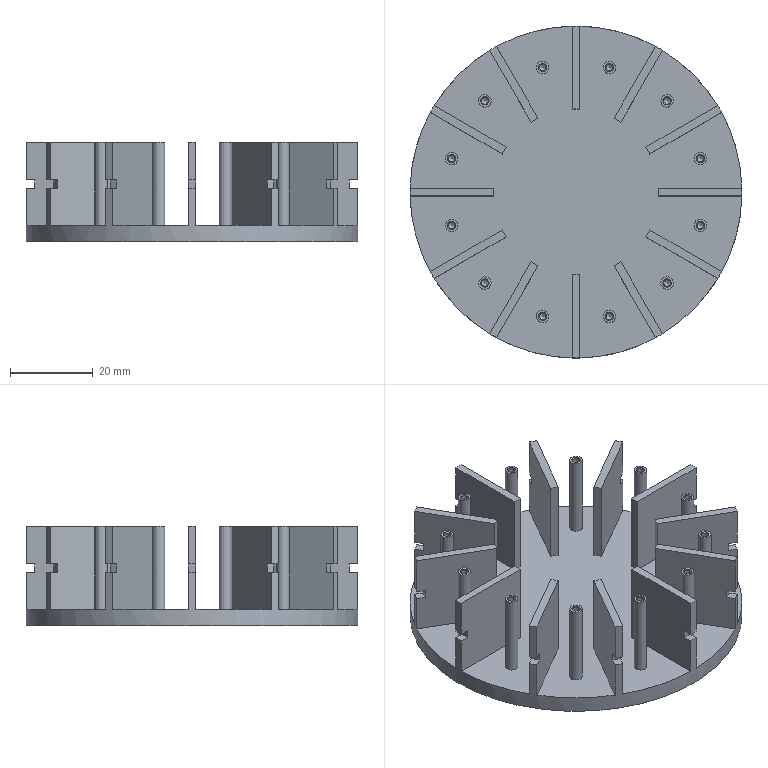Part | NX | features SIMPLE HOLE 12, SYMBOLIC_THREAD 12, DATUM_CSYS 7, EXTRUDE 6, SKETCH 6, HOLE PACKAGE 1, SWP104 1 | 1 solid | 161 faces | box 80 x 80 x 24.1 mm | volume 26700 mm3 | plane 75 | cylinder 62 | cone 24 | commonest cylinder face diameters 80 x13 1.6 x12 3 x12 40 x12 75.777 x12 50 x1